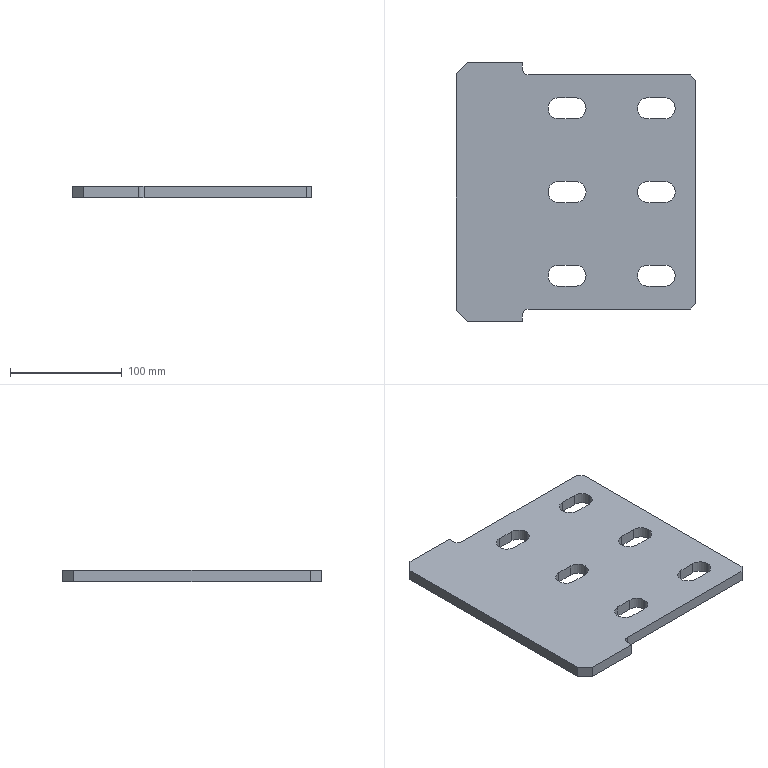Part | STEP file | 筋Plate-250×125-250 | 1 solid | 46 faces | box 215 x 232 x 10 mm | volume 429336 mm3 | plane 26 | cylinder 20 | commonest cylinder face diameters 19 x18 10 x2